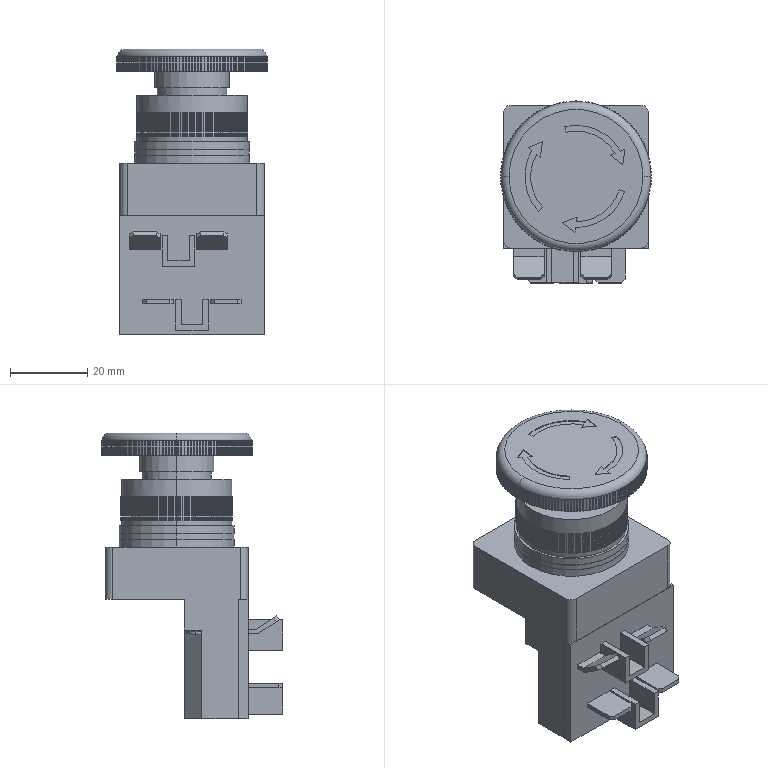Part | STEP file | Emergency hanyoung | 2 solids | 1693 faces | box 39.095 x 47.049 x 74 mm | volume 39082 mm3 | plane 1198 | cylinder 489 | torus 6 | commonest cylinder face diameters 38.7 x151 28.9 x150 39.1 x150 2.2 x4 4 x4 4.5 x4